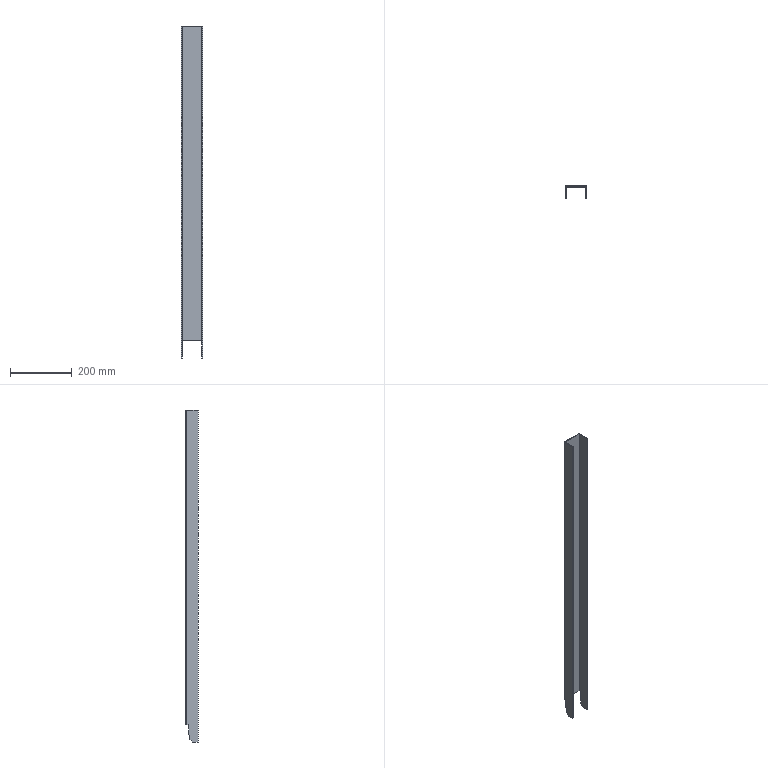Part | SolidWorks | 1 solid | 30 faces | box 70 x 40 x 1074 mm | volume 445087 mm3 | plane 26 | cylinder 4 | commonest cylinder face diameters 0.2 x2 6.2 x2
STEP:
#1=CARTESIAN_POINT('',(-31.9,-3.,-480.25));
#2=VERTEX_POINT('',#1);
#3=CARTESIAN_POINT('',(31.9,-3.,-480.25));
#4=VERTEX_POINT('',#3);
#5=CARTESIAN_POINT('',(0.,-3.,-480.25));
#6=DIRECTION('',(1.,0.,0.));
#7=VECTOR('',#6,1000.);
#8=LINE('',#5,#7);
#9=EDGE_CURVE('',#2,#4,#8,.T.);
#10=ORIENTED_EDGE('',*,*,#9,.T.);
#11=CARTESIAN_POINT('',(31.9,-3.,536.75));
#12=VERTEX_POINT('',#11);
#13=CARTESIAN_POINT('',(31.9,-3.,536.75));
#14=DIRECTION('',(0.,0.,-1.));
#15=VECTOR('',#14,1000.);
#16=LINE('',#13,#15);
#17=EDGE_CURVE('',#12,#4,#16,.T.);
#18=ORIENTED_EDGE('',*,*,#17,.F.);
#19=CARTESIAN_POINT('',(-31.9,-3.,536.75));
#20=VERTEX_POINT('',#19);
#21=CARTESIAN_POINT('',(35.,-3.,536.75));
#22=DIRECTION('',(1.,0.,0.));
#23=VECTOR('',#22,1000.);
#24=LINE('',#21,#23);
#25=EDGE_CURVE('',#20,#12,#24,.T.);
#26=ORIENTED_EDGE('',*,*,#25,.F.);
#27=CARTESIAN_POINT('',(-31.9,-3.,-536.75));
#28=DIRECTION('',(0.,0.,1.));
#29=VECTOR('',#28,1000.);
#30=LINE('',#27,#29);
#31=EDGE_CURVE('',#2,#20,#30,.T.);
#32=ORIENTED_EDGE('',*,*,#31,.F.);
#33=EDGE_LOOP('',(#10,#18,#26,#32));
#34=FACE_OUTER_BOUND('',#33,.T.);
#35=CARTESIAN_POINT('',(0.,-3.,0.));
#36=DIRECTION('',(0.,1.,0.));
#37=DIRECTION('',(0.,0.,1.));
#38=AXIS2_PLACEMENT_3D('',#35,#36,#37);
#39=PLANE('',#38);
#40=ADVANCED_FACE('',(#34),#39,.F.);
#41=CARTESIAN_POINT('',(31.9,0.,536.75));
#42=VERTEX_POINT('',#41);
#43=CARTESIAN_POINT('',(31.9,0.,-480.25));
#44=VERTEX_POINT('',#43);
#45=CARTESIAN_POINT('',(31.9,0.,536.75));
#46=DIRECTION('',(0.,0.,-1.));
#47=VECTOR('',#46,1000.);
#48=LINE('',#45,#47);
#49=EDGE_CURVE('',#42,#44,#48,.T.);
#50=ORIENTED_EDGE('',*,*,#49,.T.);
#51=CARTESIAN_POINT('',(-31.9,0.,-480.25));
#52=VERTEX_POINT('',#51);
#53=CARTESIAN_POINT('',(0.,0.,-480.25));
#54=DIRECTION('',(1.,0.,0.));
#55=VECTOR('',#54,1000.);
#56=LINE('',#53,#55);
#57=EDGE_CURVE('',#52,#44,#56,.T.);
#58=ORIENTED_EDGE('',*,*,#57,.F.);
#59=CARTESIAN_POINT('',(-31.9,0.,536.75));
#60=VERTEX_POINT('',#59);
#61=CARTESIAN_POINT('',(-31.9,0.,-536.75));
#62=DIRECTION('',(0.,0.,1.));
#63=VECTOR('',#62,1000.);
#64=LINE('',#61,#63);
#65=EDGE_CURVE('',#52,#60,#64,.T.);
#66=ORIENTED_EDGE('',*,*,#65,.T.);
#67=CARTESIAN_POINT('',(35.,0.,536.75));
#68=DIRECTION('',(1.,0.,0.));
#69=VECTOR('',#68,1000.);
#70=LINE('',#67,#69);
#71=EDGE_CURVE('',#60,#42,#70,.T.);
#72=ORIENTED_EDGE('',*,*,#71,.T.);
#73=EDGE_LOOP('',(#50,#58,#66,#72));
#74=FACE_OUTER_BOUND('',#73,.T.);
#75=CARTESIAN_POINT('',(0.,0.,0.));
#76=DIRECTION('',(0.,1.,0.));
#77=DIRECTION('',(0.,0.,1.));
#78=AXIS2_PLACEMENT_3D('',#75,#76,#77);
#79=PLANE('',#78);
#80=ADVANCED_FACE('',(#74),#79,.T.);
#81=ORIENTED_EDGE('',*,*,#65,.F.);
#82=CARTESIAN_POINT('',(-35.,-3.1,-480.25));
#83=VERTEX_POINT('',#82);
#84=CARTESIAN_POINT('',(-31.9,-3.1,-480.25));
#85=DIRECTION('',(0.,0.,-1.));
#86=DIRECTION('',(0.,-1.,0.));
#87=AXIS2_PLACEMENT_3D('',#84,#85,#86);
#88=CIRCLE('',#87,3.1);
#89=EDGE_CURVE('',#83,#52,#88,.T.);
#90=ORIENTED_EDGE('',*,*,#89,.F.);
#91=CARTESIAN_POINT('',(-35.,-3.1,536.75));
#92=VERTEX_POINT('',#91);
#93=CARTESIAN_POINT('',(-35.,-3.1,536.75));
#94=DIRECTION('',(0.,0.,1.));
#95=VECTOR('',#94,1000.);
#96=LINE('',#93,#95);
#97=EDGE_CURVE('',#83,#92,#96,.T.);
#98=ORIENTED_EDGE('',*,*,#97,.T.);
#99=CARTESIAN_POINT('',(-31.9,-3.1,536.75));
#100=DIRECTION('',(0.,0.,1.));
#101=DIRECTION('',(-1.,0.,0.));
#102=AXIS2_PLACEMENT_3D('',#99,#100,#101);
#103=CIRCLE('',#102,3.1);
#104=EDGE_CURVE('',#60,#92,#103,.T.);
#105=ORIENTED_EDGE('',*,*,#104,.F.);
#106=EDGE_LOOP('',(#81,#90,#98,#105));
#107=FACE_OUTER_BOUND('',#106,.T.);
#108=CARTESIAN_POINT('',(-31.9,-3.1,-536.75));
#109=DIRECTION('',(0.,0.,-1.));
#110=DIRECTION('',(-1.,0.,0.));
#111=AXIS2_PLACEMENT_3D('',#108,#109,#110);
#112=CYLINDRICAL_SURFACE('',#111,3.1);
#113=ADVANCED_FACE('',(#107),#112,.T.);
#114=CARTESIAN_POINT('',(-32.,-3.1,-480.25));
#115=VERTEX_POINT('',#114);
#116=CARTESIAN_POINT('',(-31.9,-3.1,-480.25));
#117=DIRECTION('',(0.,0.,-1.));
#118=DIRECTION('',(-1.,0.,0.));
#119=AXIS2_PLACEMENT_3D('',#116,#117,#118);
#120=CIRCLE('',#119,0.1);
#121=EDGE_CURVE('',#115,#2,#120,.T.);
#122=ORIENTED_EDGE('',*,*,#121,.T.);
#123=ORIENTED_EDGE('',*,*,#31,.T.);
#124=CARTESIAN_POINT('',(-32.,-3.1,536.75));
#125=VERTEX_POINT('',#124);
#126=CARTESIAN_POINT('',(-31.9,-3.1,536.75));
#127=DIRECTION('',(0.,0.,1.));
#128=DIRECTION('',(-1.,0.,0.));
#129=AXIS2_PLACEMENT_3D('',#126,#127,#128);
#130=CIRCLE('',#129,0.1);
#131=EDGE_CURVE('',#20,#125,#130,.T.);
#132=ORIENTED_EDGE('',*,*,#131,.T.);
#133=CARTESIAN_POINT('',(-32.,-3.1,536.75));
#134=DIRECTION('',(0.,0.,-1.));
#135=VECTOR('',#134,1000.);
#136=LINE('',#133,#135);
#137=EDGE_CURVE('',#125,#115,#136,.T.);
#138=ORIENTED_EDGE('',*,*,#137,.T.);
#139=EDGE_LOOP('',(#122,#123,#132,#138));
#140=FACE_OUTER_BOUND('',#139,.T.);
#141=CARTESIAN_POINT('',(-31.9,-3.1,-536.75));
#142=DIRECTION('',(0.,0.,-1.));
#143=DIRECTION('',(-1.,0.,0.));
#144=AXIS2_PLACEMENT_3D('',#141,#142,#143);
#145=CYLINDRICAL_SURFACE('',#144,0.1);
#146=ADVANCED_FACE('',(#140),#145,.F.);
#147=CARTESIAN_POINT('',(-32.,-21.55,-536.75));
#148=VERTEX_POINT('',#147);
#149=CARTESIAN_POINT('',(-35.,-21.55,-536.75));
#150=VERTEX_POINT('',#149);
#151=CARTESIAN_POINT('',(-32.,-21.55,-536.75));
#152=DIRECTION('',(-1.,0.,0.));
#153=VECTOR('',#152,1000.);
#154=LINE('',#151,#153);
#155=EDGE_CURVE('',#148,#150,#154,.T.);
#156=ORIENTED_EDGE('',*,*,#155,.F.);
#157=CARTESIAN_POINT('',(-32.,-40.,-536.75));
#158=VERTEX_POINT('',#157);
#159=CARTESIAN_POINT('',(-32.,-40.,-536.75));
#160=DIRECTION('',(0.,-1.,0.));
#161=VECTOR('',#160,1000.);
#162=LINE('',#159,#161);
#163=EDGE_CURVE('',#148,#158,#162,.T.);
#164=ORIENTED_EDGE('',*,*,#163,.T.);
#165=CARTESIAN_POINT('',(-35.,-40.,-536.75));
#166=VERTEX_POINT('',#165);
#167=CARTESIAN_POINT('',(-35.,-40.,-536.75));
#168=DIRECTION('',(1.,0.,0.));
#169=VECTOR('',#168,1000.);
#170=LINE('',#167,#169);
#171=EDGE_CURVE('',#166,#158,#170,.T.);
#172=ORIENTED_EDGE('',*,*,#171,.F.);
#173=CARTESIAN_POINT('',(-35.,0.,-536.75));
#174=DIRECTION('',(0.,-1.,0.));
#175=VECTOR('',#174,1000.);
#176=LINE('',#173,#175);
#177=EDGE_CURVE('',#150,#166,#176,.T.);
#178=ORIENTED_EDGE('',*,*,#177,.F.);
#179=EDGE_LOOP('',(#156,#164,#172,#178));
#180=FACE_OUTER_BOUND('',#179,.T.);
#181=CARTESIAN_POINT('',(-35.,-40.,-536.75));
#182=DIRECTION('',(0.,0.,1.));
#183=DIRECTION('',(1.,0.,0.));
#184=AXIS2_PLACEMENT_3D('',#181,#182,#183);
#185=PLANE('',#184);
#186=ADVANCED_FACE('',(#180),#185,.F.);
#187=CARTESIAN_POINT('',(-35.,-7.501,-480.25));
#188=VERTEX_POINT('',#187);
#189=CARTESIAN_POINT('',(-35.,0.,-480.25));
#190=DIRECTION('',(0.,-1.,0.));
#191=VECTOR('',#190,1000.);
#192=LINE('',#189,#191);
#193=EDGE_CURVE('',#83,#188,#192,.T.);
#194=ORIENTED_EDGE('',*,*,#193,.T.);
#195=CARTESIAN_POINT('',(-35.,-7.501,-484.727));
#196=VERTEX_POINT('',#195);
#197=CARTESIAN_POINT('',(-35.,-7.501,0.));
#198=DIRECTION('',(0.,0.,-1.));
#199=VECTOR('',#198,1000.);
#200=LINE('',#197,#199);
#201=EDGE_CURVE('',#188,#196,#200,.T.);
#202=ORIENTED_EDGE('',*,*,#201,.T.);
#203=CARTESIAN_POINT('',(-35.,-12.028,-527.795));
#204=VERTEX_POINT('',#203);
#205=CARTESIAN_POINT('',(-35.,42.971,-4.516));
#206=DIRECTION('',(0.,-0.1045,-0.9945));
#207=VECTOR('',#206,1000.);
#208=LINE('',#205,#207);
#209=EDGE_CURVE('',#196,#204,#208,.T.);
#210=ORIENTED_EDGE('',*,*,#209,.T.);
#211=CARTESIAN_POINT('',(-35.,257.756,-274.084));
#212=DIRECTION('',(0.,-0.7285,-0.6851));
#213=VECTOR('',#212,1000.);
#214=LINE('',#211,#213);
#215=EDGE_CURVE('',#204,#150,#214,.T.);
#216=ORIENTED_EDGE('',*,*,#215,.T.);
#217=ORIENTED_EDGE('',*,*,#177,.T.);
#218=CARTESIAN_POINT('',(-35.,-40.,536.75));
#219=VERTEX_POINT('',#218);
#220=CARTESIAN_POINT('',(-35.,-40.,0.));
#221=DIRECTION('',(0.,0.,1.));
#222=VECTOR('',#221,1000.);
#223=LINE('',#220,#222);
#224=EDGE_CURVE('',#166,#219,#223,.T.);
#225=ORIENTED_EDGE('',*,*,#224,.T.);
#226=CARTESIAN_POINT('',(-35.,0.,536.75));
#227=DIRECTION('',(0.,1.,0.));
#228=VECTOR('',#227,1000.);
#229=LINE('',#226,#228);
#230=EDGE_CURVE('',#219,#92,#229,.T.);
#231=ORIENTED_EDGE('',*,*,#230,.T.);
#232=ORIENTED_EDGE('',*,*,#97,.F.);
#233=EDGE_LOOP('',(#194,#202,#210,#216,#217,#225,#231,#232));
#234=FACE_OUTER_BOUND('',#233,.T.);
#235=CARTESIAN_POINT('',(-35.,0.,0.));
#236=DIRECTION('',(1.,0.,0.));
#237=DIRECTION('',(0.,1.,0.));
#238=AXIS2_PLACEMENT_3D('',#235,#236,#237);
#239=PLANE('',#238);
#240=ADVANCED_FACE('',(#234),#239,.F.);
#241=CARTESIAN_POINT('',(-32.,-7.501,-480.25));
#242=VERTEX_POINT('',#241);
#243=CARTESIAN_POINT('',(-32.,-7.501,-484.727));
#244=VERTEX_POINT('',#243);
#245=CARTESIAN_POINT('',(-32.,-7.501,0.));
#246=DIRECTION('',(0.,0.,-1.));
#247=VECTOR('',#246,1000.);
#248=LINE('',#245,#247);
#249=EDGE_CURVE('',#242,#244,#248,.T.);
#250=ORIENTED_EDGE('',*,*,#249,.F.);
#251=CARTESIAN_POINT('',(-32.,0.,-480.25));
#252=DIRECTION('',(0.,-1.,0.));
#253=VECTOR('',#252,1000.);
#254=LINE('',#251,#253);
#255=EDGE_CURVE('',#115,#242,#254,.T.);
#256=ORIENTED_EDGE('',*,*,#255,.F.);
#257=ORIENTED_EDGE('',*,*,#137,.F.);
#258=CARTESIAN_POINT('',(-32.,-40.,536.75));
#259=VERTEX_POINT('',#258);
#260=CARTESIAN_POINT('',(-32.,-3.,536.75));
#261=DIRECTION('',(0.,1.,0.));
#262=VECTOR('',#261,1000.);
#263=LINE('',#260,#262);
#264=EDGE_CURVE('',#259,#125,#263,.T.);
#265=ORIENTED_EDGE('',*,*,#264,.F.);
#266=CARTESIAN_POINT('',(-32.,-40.,536.75));
#267=DIRECTION('',(0.,0.,1.));
#268=VECTOR('',#267,1000.);
#269=LINE('',#266,#268);
#270=EDGE_CURVE('',#158,#259,#269,.T.);
#271=ORIENTED_EDGE('',*,*,#270,.F.);
#272=ORIENTED_EDGE('',*,*,#163,.F.);
#273=CARTESIAN_POINT('',(-32.,-12.028,-527.795));
#274=VERTEX_POINT('',#273);
#275=CARTESIAN_POINT('',(-32.,257.756,-274.084));
#276=DIRECTION('',(0.,-0.7285,-0.6851));
#277=VECTOR('',#276,1000.);
#278=LINE('',#275,#277);
#279=EDGE_CURVE('',#274,#148,#278,.T.);
#280=ORIENTED_EDGE('',*,*,#279,.F.);
#281=CARTESIAN_POINT('',(-32.,42.971,-4.516));
#282=DIRECTION('',(0.,-0.1045,-0.9945));
#283=VECTOR('',#282,1000.);
#284=LINE('',#281,#283);
#285=EDGE_CURVE('',#244,#274,#284,.T.);
#286=ORIENTED_EDGE('',*,*,#285,.F.);
#287=EDGE_LOOP('',(#250,#256,#257,#265,#271,#272,#280,#286));
#288=FACE_OUTER_BOUND('',#287,.T.);
#289=CARTESIAN_POINT('',(-32.,0.,0.));
#290=DIRECTION('',(1.,0.,0.));
#291=DIRECTION('',(0.,1.,0.));
#292=AXIS2_PLACEMENT_3D('',#289,#290,#291);
#293=PLANE('',#292);
#294=ADVANCED_FACE('',(#288),#293,.T.);
#295=CARTESIAN_POINT('',(35.,-3.1,536.75));
#296=VERTEX_POINT('',#295);
#297=CARTESIAN_POINT('',(35.,-3.1,-480.25));
#298=VERTEX_POINT('',#297);
#299=CARTESIAN_POINT('',(35.,-3.1,-536.75));
#300=DIRECTION('',(0.,0.,-1.));
#301=VECTOR('',#300,1000.);
#302=LINE('',#299,#301);
#303=EDGE_CURVE('',#296,#298,#302,.T.);
#304=ORIENTED_EDGE('',*,*,#303,.T.);
#305=CARTESIAN_POINT('',(31.9,-3.1,-480.25));
#306=DIRECTION('',(0.,0.,-1.));
#307=DIRECTION('',(1.,0.,0.));
#308=AXIS2_PLACEMENT_3D('',#305,#306,#307);
#309=CIRCLE('',#308,3.1);
#310=EDGE_CURVE('',#44,#298,#309,.T.);
#311=ORIENTED_EDGE('',*,*,#310,.F.);
#312=ORIENTED_EDGE('',*,*,#49,.F.);
#313=CARTESIAN_POINT('',(31.9,-3.1,536.75));
#314=DIRECTION('',(0.,0.,1.));
#315=DIRECTION('',(1.,0.,0.));
#316=AXIS2_PLACEMENT_3D('',#313,#314,#315);
#317=CIRCLE('',#316,3.1);
#318=EDGE_CURVE('',#296,#42,#317,.T.);
#319=ORIENTED_EDGE('',*,*,#318,.F.);
#320=EDGE_LOOP('',(#304,#311,#312,#319));
#321=FACE_OUTER_BOUND('',#320,.T.);
#322=CARTESIAN_POINT('',(31.9,-3.1,536.75));
#323=DIRECTION('',(0.,0.,1.));
#324=DIRECTION('',(1.,0.,0.));
#325=AXIS2_PLACEMENT_3D('',#322,#323,#324);
#326=CYLINDRICAL_SURFACE('',#325,3.1);
#327=ADVANCED_FACE('',(#321),#326,.T.);
#328=CARTESIAN_POINT('',(32.,-3.1,-480.25));
#329=VERTEX_POINT('',#328);
#330=CARTESIAN_POINT('',(31.9,-3.1,-480.25));
#331=DIRECTION('',(0.,0.,-1.));
#332=DIRECTION('',(0.,-1.,0.));
#333=AXIS2_PLACEMENT_3D('',#330,#331,#332);
#334=CIRCLE('',#333,0.1);
#335=EDGE_CURVE('',#4,#329,#334,.T.);
#336=ORIENTED_EDGE('',*,*,#335,.T.);
#337=CARTESIAN_POINT('',(32.,-3.1,536.75));
#338=VERTEX_POINT('',#337);
#339=CARTESIAN_POINT('',(32.,-3.1,-536.75));
#340=DIRECTION('',(0.,0.,1.));
#341=VECTOR('',#340,1000.);
#342=LINE('',#339,#341);
#343=EDGE_CURVE('',#329,#338,#342,.T.);
#344=ORIENTED_EDGE('',*,*,#343,.T.);
#345=CARTESIAN_POINT('',(31.9,-3.1,536.75));
#346=DIRECTION('',(0.,0.,1.));
#347=DIRECTION('',(1.,0.,0.));
#348=AXIS2_PLACEMENT_3D('',#345,#346,#347);
#349=CIRCLE('',#348,0.1);
#350=EDGE_CURVE('',#338,#12,#349,.T.);
#351=ORIENTED_EDGE('',*,*,#350,.T.);
#352=ORIENTED_EDGE('',*,*,#17,.T.);
#353=EDGE_LOOP('',(#336,#344,#351,#352));
#354=FACE_OUTER_BOUND('',#353,.T.);
#355=CARTESIAN_POINT('',(31.9,-3.1,536.75));
#356=DIRECTION('',(0.,0.,1.));
#357=DIRECTION('',(1.,0.,0.));
#358=AXIS2_PLACEMENT_3D('',#355,#356,#357);
#359=CYLINDRICAL_SURFACE('',#358,0.1);
#360=ADVANCED_FACE('',(#354),#359,.F.);
#361=CARTESIAN_POINT('',(32.,-21.55,-536.75));
#362=VERTEX_POINT('',#361);
#363=CARTESIAN_POINT('',(35.,-21.55,-536.75));
#364=VERTEX_POINT('',#363);
#365=CARTESIAN_POINT('',(32.,-21.55,-536.75));
#366=DIRECTION('',(1.,0.,0.));
#367=VECTOR('',#366,1000.);
#368=LINE('',#365,#367);
#369=EDGE_CURVE('',#362,#364,#368,.T.);
#370=ORIENTED_EDGE('',*,*,#369,.T.);
#371=CARTESIAN_POINT('',(35.,-40.,-536.75));
#372=VERTEX_POINT('',#371);
#373=CARTESIAN_POINT('',(35.,0.,-536.75));
#374=DIRECTION('',(0.,1.,0.));
#375=VECTOR('',#374,1000.);
#376=LINE('',#373,#375);
#377=EDGE_CURVE('',#372,#364,#376,.T.);
#378=ORIENTED_EDGE('',*,*,#377,.F.);
#379=CARTESIAN_POINT('',(32.,-40.,-536.75));
#380=VERTEX_POINT('',#379);
#381=CARTESIAN_POINT('',(35.,-40.,-536.75));
#382=DIRECTION('',(-1.,0.,0.));
#383=VECTOR('',#382,1000.);
#384=LINE('',#381,#383);
#385=EDGE_CURVE('',#372,#380,#384,.T.);
#386=ORIENTED_EDGE('',*,*,#385,.T.);
#387=CARTESIAN_POINT('',(32.,-3.,-536.75));
#388=DIRECTION('',(0.,1.,0.));
#389=VECTOR('',#388,1000.);
#390=LINE('',#387,#389);
#391=EDGE_CURVE('',#380,#362,#390,.T.);
#392=ORIENTED_EDGE('',*,*,#391,.T.);
#393=EDGE_LOOP('',(#370,#378,#386,#392));
#394=FACE_OUTER_BOUND('',#393,.T.);
#395=CARTESIAN_POINT('',(35.,-3.,-536.75));
#396=DIRECTION('',(0.,0.,1.));
#397=DIRECTION('',(1.,0.,0.));
#398=AXIS2_PLACEMENT_3D('',#395,#396,#397);
#399=PLANE('',#398);
#400=ADVANCED_FACE('',(#394),#399,.F.);
#401=CARTESIAN_POINT('',(35.,-12.028,-527.795));
#402=VERTEX_POINT('',#401);
#403=CARTESIAN_POINT('',(35.,257.756,-274.084));
#404=DIRECTION('',(0.,0.7285,0.6851));
#405=VECTOR('',#404,1000.);
#406=LINE('',#403,#405);
#407=EDGE_CURVE('',#364,#402,#406,.T.);
#408=ORIENTED_EDGE('',*,*,#407,.T.);
#409=CARTESIAN_POINT('',(35.,-7.501,-484.727));
#410=VERTEX_POINT('',#409);
#411=CARTESIAN_POINT('',(35.,42.971,-4.516));
#412=DIRECTION('',(0.,0.1045,0.9945));
#413=VECTOR('',#412,1000.);
#414=LINE('',#411,#413);
#415=EDGE_CURVE('',#402,#410,#414,.T.);
#416=ORIENTED_EDGE('',*,*,#415,.T.);
#417=CARTESIAN_POINT('',(35.,-7.501,-480.25));
#418=VERTEX_POINT('',#417);
#419=CARTESIAN_POINT('',(35.,-7.501,0.));
#420=DIRECTION('',(0.,0.,1.));
#421=VECTOR('',#420,1000.);
#422=LINE('',#419,#421);
#423=EDGE_CURVE('',#410,#418,#422,.T.);
#424=ORIENTED_EDGE('',*,*,#423,.T.);
#425=CARTESIAN_POINT('',(35.,0.,-480.25));
#426=DIRECTION('',(0.,1.,0.));
#427=VECTOR('',#426,1000.);
#428=LINE('',#425,#427);
#429=EDGE_CURVE('',#418,#298,#428,.T.);
#430=ORIENTED_EDGE('',*,*,#429,.T.);
#431=ORIENTED_EDGE('',*,*,#303,.F.);
#432=CARTESIAN_POINT('',(35.,-40.,536.75));
#433=VERTEX_POINT('',#432);
#434=CARTESIAN_POINT('',(35.,0.,536.75));
#435=DIRECTION('',(0.,-1.,0.));
#436=VECTOR('',#435,1000.);
#437=LINE('',#434,#436);
#438=EDGE_CURVE('',#296,#433,#437,.T.);
#439=ORIENTED_EDGE('',*,*,#438,.T.);
#440=CARTESIAN_POINT('',(35.,-40.,0.));
#441=DIRECTION('',(0.,0.,-1.));
#442=VECTOR('',#441,1000.);
#443=LINE('',#440,#442);
#444=EDGE_CURVE('',#433,#372,#443,.T.);
#445=ORIENTED_EDGE('',*,*,#444,.T.);
#446=ORIENTED_EDGE('',*,*,#377,.T.);
#447=EDGE_LOOP('',(#408,#416,#424,#430,#431,#439,#445,#446));
#448=FACE_OUTER_BOUND('',#447,.T.);
#449=CARTESIAN_POINT('',(35.,0.,0.));
#450=DIRECTION('',(-1.,0.,0.));
#451=DIRECTION('',(0.,-1.,0.));
#452=AXIS2_PLACEMENT_3D('',#449,#450,#451);
#453=PLANE('',#452);
#454=ADVANCED_FACE('',(#448),#453,.F.);
#455=CARTESIAN_POINT('',(32.,-12.028,-527.795));
#456=VERTEX_POINT('',#455);
#457=CARTESIAN_POINT('',(32.,-7.501,-484.727));
#458=VERTEX_POINT('',#457);
#459=CARTESIAN_POINT('',(32.,42.971,-4.516));
#460=DIRECTION('',(0.,0.1045,0.9945));
#461=VECTOR('',#460,1000.);
#462=LINE('',#459,#461);
#463=EDGE_CURVE('',#456,#458,#462,.T.);
#464=ORIENTED_EDGE('',*,*,#463,.F.);
#465=CARTESIAN_POINT('',(32.,257.756,-274.084));
#466=DIRECTION('',(0.,0.7285,0.6851));
#467=VECTOR('',#466,1000.);
#468=LINE('',#465,#467);
#469=EDGE_CURVE('',#362,#456,#468,.T.);
#470=ORIENTED_EDGE('',*,*,#469,.F.);
#471=ORIENTED_EDGE('',*,*,#391,.F.);
#472=CARTESIAN_POINT('',(32.,-40.,536.75));
#473=VERTEX_POINT('',#472);
#474=CARTESIAN_POINT('',(32.,-40.,-536.75));
#475=DIRECTION('',(0.,0.,-1.));
#476=VECTOR('',#475,1000.);
#477=LINE('',#474,#476);
#478=EDGE_CURVE('',#473,#380,#477,.T.);
#479=ORIENTED_EDGE('',*,*,#478,.F.);
#480=CARTESIAN_POINT('',(32.,-40.,536.75));
#481=DIRECTION('',(0.,-1.,0.));
#482=VECTOR('',#481,1000.);
#483=LINE('',#480,#482);
#484=EDGE_CURVE('',#338,#473,#483,.T.);
#485=ORIENTED_EDGE('',*,*,#484,.F.);
#486=ORIENTED_EDGE('',*,*,#343,.F.);
#487=CARTESIAN_POINT('',(32.,-7.501,-480.25));
#488=VERTEX_POINT('',#487);
#489=CARTESIAN_POINT('',(32.,0.,-480.25));
#490=DIRECTION('',(0.,1.,0.));
#491=VECTOR('',#490,1000.);
#492=LINE('',#489,#491);
#493=EDGE_CURVE('',#488,#329,#492,.T.);
#494=ORIENTED_EDGE('',*,*,#493,.F.);
#495=CARTESIAN_POINT('',(32.,-7.501,0.));
#496=DIRECTION('',(0.,0.,1.));
#497=VECTOR('',#496,1000.);
#498=LINE('',#495,#497);
#499=EDGE_CURVE('',#458,#488,#498,.T.);
#500=ORIENTED_EDGE('',*,*,#499,.F.);
#501=EDGE_LOOP('',(#464,#470,#471,#479,#485,#486,#494,#500));
#502=FACE_OUTER_BOUND('',#501,.T.);
#503=CARTESIAN_POINT('',(32.,0.,0.));
#504=DIRECTION('',(-1.,0.,0.));
#505=DIRECTION('',(0.,-1.,0.));
#506=AXIS2_PLACEMENT_3D('',#503,#504,#505);
#507=PLANE('',#506);
#508=ADVANCED_FACE('',(#502),#507,.T.);
#509=ORIENTED_EDGE('',*,*,#25,.T.);
#510=CARTESIAN_POINT('',(31.9,-3.,536.75));
#511=DIRECTION('',(0.,1.,0.));
#512=VECTOR('',#511,1000.);
#513=LINE('',#510,#512);
#514=EDGE_CURVE('',#12,#42,#513,.T.);
#515=ORIENTED_EDGE('',*,*,#514,.T.);
#516=ORIENTED_EDGE('',*,*,#71,.F.);
#517=CARTESIAN_POINT('',(-31.9,-3.,536.75));
#518=DIRECTION('',(0.,1.,0.));
#519=VECTOR('',#518,1000.);
#520=LINE('',#517,#519);
#521=EDGE_CURVE('',#20,#60,#520,.T.);
#522=ORIENTED_EDGE('',*,*,#521,.F.);
#523=EDGE_LOOP('',(#509,#515,#516,#522));
#524=FACE_OUTER_BOUND('',#523,.T.);
#525=CARTESIAN_POINT('',(35.,-3.,536.75));
#526=DIRECTION('',(0.,0.,1.));
#527=DIRECTION('',(1.,0.,0.));
#528=AXIS2_PLACEMENT_3D('',#525,#526,#527);
#529=PLANE('',#528);
#530=ADVANCED_FACE('',(#524),#529,.T.);
#531=CARTESIAN_POINT('',(-35.,-3.1,536.75));
#532=DIRECTION('',(-1.,0.,0.));
#533=VECTOR('',#532,1000.);
#534=LINE('',#531,#533);
#535=EDGE_CURVE('',#125,#92,#534,.T.);
#536=ORIENTED_EDGE('',*,*,#535,.F.);
#537=ORIENTED_EDGE('',*,*,#131,.F.);
#538=ORIENTED_EDGE('',*,*,#521,.T.);
#539=ORIENTED_EDGE('',*,*,#104,.T.);
#540=EDGE_LOOP('',(#536,#537,#538,#539));
#541=FACE_OUTER_BOUND('',#540,.T.);
#542=CARTESIAN_POINT('',(-31.9,-3.1,536.75));
#543=DIRECTION('',(0.,0.,1.));
#544=DIRECTION('',(1.,0.,0.));
#545=AXIS2_PLACEMENT_3D('',#542,#543,#544);
#546=PLANE('',#545);
#547=ADVANCED_FACE('',(#541),#546,.T.);
#548=ORIENTED_EDGE('',*,*,#535,.T.);
#549=ORIENTED_EDGE('',*,*,#230,.F.);
#550=CARTESIAN_POINT('',(-35.,-40.,536.75));
#551=DIRECTION('',(1.,0.,0.));
#552=VECTOR('',#551,1000.);
#553=LINE('',#550,#552);
#554=EDGE_CURVE('',#219,#259,#553,.T.);
#555=ORIENTED_EDGE('',*,*,#554,.T.);
#556=ORIENTED_EDGE('',*,*,#264,.T.);
#557=EDGE_LOOP('',(#548,#549,#555,#556));
#558=FACE_OUTER_BOUND('',#557,.T.);
#559=CARTESIAN_POINT('',(-35.,-3.,536.75));
#560=DIRECTION('',(0.,0.,-1.));
#561=DIRECTION('',(-1.,0.,0.));
#562=AXIS2_PLACEMENT_3D('',#559,#560,#561);
#563=PLANE('',#562);
#564=ADVANCED_FACE('',(#558),#563,.F.);
#565=ORIENTED_EDGE('',*,*,#270,.T.);
#566=ORIENTED_EDGE('',*,*,#554,.F.);
#567=ORIENTED_EDGE('',*,*,#224,.F.);
#568=ORIENTED_EDGE('',*,*,#171,.T.);
#569=EDGE_LOOP('',(#565,#566,#567,#568));
#570=FACE_OUTER_BOUND('',#569,.T.);
#571=CARTESIAN_POINT('',(-35.,-40.,536.75));
#572=DIRECTION('',(0.,1.,0.));
#573=DIRECTION('',(-1.,0.,0.));
#574=AXIS2_PLACEMENT_3D('',#571,#572,#573);
#575=PLANE('',#574);
#576=ADVANCED_FACE('',(#570),#575,.F.);
#577=ORIENTED_EDGE('',*,*,#350,.F.);
#578=CARTESIAN_POINT('',(32.,-3.1,536.75));
#579=DIRECTION('',(1.,0.,0.));
#580=VECTOR('',#579,1000.);
#581=LINE('',#578,#580);
#582=EDGE_CURVE('',#338,#296,#581,.T.);
#583=ORIENTED_EDGE('',*,*,#582,.T.);
#584=ORIENTED_EDGE('',*,*,#318,.T.);
#585=ORIENTED_EDGE('',*,*,#514,.F.);
#586=EDGE_LOOP('',(#577,#583,#584,#585));
#587=FACE_OUTER_BOUND('',#586,.T.);
#588=CARTESIAN_POINT('',(31.9,-3.1,536.75));
#589=DIRECTION('',(0.,0.,-1.));
#590=DIRECTION('',(-1.,0.,0.));
#591=AXIS2_PLACEMENT_3D('',#588,#589,#590);
#592=PLANE('',#591);
#593=ADVANCED_FACE('',(#587),#592,.F.);
#594=ORIENTED_EDGE('',*,*,#582,.F.);
#595=ORIENTED_EDGE('',*,*,#484,.T.);
#596=CARTESIAN_POINT('',(35.,-40.,536.75));
#597=DIRECTION('',(-1.,0.,0.));
#598=VECTOR('',#597,1000.);
#599=LINE('',#596,#598);
#600=EDGE_CURVE('',#433,#473,#599,.T.);
#601=ORIENTED_EDGE('',*,*,#600,.F.);
#602=ORIENTED_EDGE('',*,*,#438,.F.);
#603=EDGE_LOOP('',(#594,#595,#601,#602));
#604=FACE_OUTER_BOUND('',#603,.T.);
#605=CARTESIAN_POINT('',(35.,-40.,536.75));
#606=DIRECTION('',(0.,0.,-1.));
#607=DIRECTION('',(-1.,0.,0.));
#608=AXIS2_PLACEMENT_3D('',#605,#606,#607);
#609=PLANE('',#608);
#610=ADVANCED_FACE('',(#604),#609,.F.);
#611=ORIENTED_EDGE('',*,*,#478,.T.);
#612=ORIENTED_EDGE('',*,*,#385,.F.);
#613=ORIENTED_EDGE('',*,*,#444,.F.);
#614=ORIENTED_EDGE('',*,*,#600,.T.);
#615=EDGE_LOOP('',(#611,#612,#613,#614));
#616=FACE_OUTER_BOUND('',#615,.T.);
#617=CARTESIAN_POINT('',(35.,-40.,-536.75));
#618=DIRECTION('',(0.,1.,0.));
#619=DIRECTION('',(-1.,0.,0.));
#620=AXIS2_PLACEMENT_3D('',#617,#618,#619);
#621=PLANE('',#620);
#622=ADVANCED_FACE('',(#616),#621,.F.);
#623=CARTESIAN_POINT('',(-32.,-3.1,-480.25));
#624=DIRECTION('',(-1.,0.,0.));
#625=VECTOR('',#624,1000.);
#626=LINE('',#623,#625);
#627=EDGE_CURVE('',#115,#83,#626,.T.);
#628=ORIENTED_EDGE('',*,*,#627,.F.);
#629=ORIENTED_EDGE('',*,*,#255,.T.);
#630=CARTESIAN_POINT('',(-32.,-7.501,-480.25));
#631=DIRECTION('',(-1.,0.,0.));
#632=VECTOR('',#631,1000.);
#633=LINE('',#630,#632);
#634=EDGE_CURVE('',#242,#188,#633,.T.);
#635=ORIENTED_EDGE('',*,*,#634,.T.);
#636=ORIENTED_EDGE('',*,*,#193,.F.);
#637=EDGE_LOOP('',(#628,#629,#635,#636));
#638=FACE_OUTER_BOUND('',#637,.T.);
#639=CARTESIAN_POINT('',(-32.,0.,-480.25));
#640=DIRECTION('',(0.,0.,1.));
#641=DIRECTION('',(0.,-1.,0.));
#642=AXIS2_PLACEMENT_3D('',#639,#640,#641);
#643=PLANE('',#642);
#644=ADVANCED_FACE('',(#638),#643,.F.);
#645=ORIENTED_EDGE('',*,*,#634,.F.);
#646=ORIENTED_EDGE('',*,*,#249,.T.);
#647=CARTESIAN_POINT('',(-32.,-7.501,-484.727));
#648=DIRECTION('',(-1.,0.,0.));
#649=VECTOR('',#648,1000.);
#650=LINE('',#647,#649);
#651=EDGE_CURVE('',#244,#196,#650,.T.);
#652=ORIENTED_EDGE('',*,*,#651,.T.);
#653=ORIENTED_EDGE('',*,*,#201,.F.);
#654=EDGE_LOOP('',(#645,#646,#652,#653));
#655=FACE_OUTER_BOUND('',#654,.T.);
#656=CARTESIAN_POINT('',(-32.,-7.501,0.));
#657=DIRECTION('',(0.,-1.,0.));
#658=DIRECTION('',(0.,0.,-1.));
#659=AXIS2_PLACEMENT_3D('',#656,#657,#658);
#660=PLANE('',#659);
#661=ADVANCED_FACE('',(#655),#660,.F.);
#662=ORIENTED_EDGE('',*,*,#651,.F.);
#663=ORIENTED_EDGE('',*,*,#285,.T.);
#664=CARTESIAN_POINT('',(-32.,-12.028,-527.795));
#665=DIRECTION('',(-1.,0.,0.));
#666=VECTOR('',#665,1000.);
#667=LINE('',#664,#666);
#668=EDGE_CURVE('',#274,#204,#667,.T.);
#669=ORIENTED_EDGE('',*,*,#668,.T.);
#670=ORIENTED_EDGE('',*,*,#209,.F.);
#671=EDGE_LOOP('',(#662,#663,#669,#670));
#672=FACE_OUTER_BOUND('',#671,.T.);
#673=CARTESIAN_POINT('',(-32.,42.971,-4.516));
#674=DIRECTION('',(0.,-0.9945,0.1045));
#675=DIRECTION('',(0.,-0.1045,-0.9945));
#676=AXIS2_PLACEMENT_3D('',#673,#674,#675);
#677=PLANE('',#676);
#678=ADVANCED_FACE('',(#672),#677,.F.);
#679=ORIENTED_EDGE('',*,*,#279,.T.);
#680=ORIENTED_EDGE('',*,*,#155,.T.);
#681=ORIENTED_EDGE('',*,*,#215,.F.);
#682=ORIENTED_EDGE('',*,*,#668,.F.);
#683=EDGE_LOOP('',(#679,#680,#681,#682));
#684=FACE_OUTER_BOUND('',#683,.T.);
#685=CARTESIAN_POINT('',(-32.,257.756,-274.084));
#686=DIRECTION('',(0.,-0.6851,0.7285));
#687=DIRECTION('',(0.,-0.7285,-0.6851));
#688=AXIS2_PLACEMENT_3D('',#685,#686,#687);
#689=PLANE('',#688);
#690=ADVANCED_FACE('',(#684),#689,.F.);
#691=ORIENTED_EDGE('',*,*,#369,.F.);
#692=ORIENTED_EDGE('',*,*,#469,.T.);
#693=CARTESIAN_POINT('',(32.,-12.028,-527.795));
#694=DIRECTION('',(1.,0.,0.));
#695=VECTOR('',#694,1000.);
#696=LINE('',#693,#695);
#697=EDGE_CURVE('',#456,#402,#696,.T.);
#698=ORIENTED_EDGE('',*,*,#697,.T.);
#699=ORIENTED_EDGE('',*,*,#407,.F.);
#700=EDGE_LOOP('',(#691,#692,#698,#699));
#701=FACE_OUTER_BOUND('',#700,.T.);
#702=CARTESIAN_POINT('',(32.,257.756,-274.084));
#703=DIRECTION('',(0.,-0.6851,0.7285));
#704=DIRECTION('',(0.,0.7285,0.6851));
#705=AXIS2_PLACEMENT_3D('',#702,#703,#704);
#706=PLANE('',#705);
#707=ADVANCED_FACE('',(#701),#706,.F.);
#708=ORIENTED_EDGE('',*,*,#697,.F.);
#709=ORIENTED_EDGE('',*,*,#463,.T.);
#710=CARTESIAN_POINT('',(32.,-7.501,-484.727));
#711=DIRECTION('',(1.,0.,0.));
#712=VECTOR('',#711,1000.);
#713=LINE('',#710,#712);
#714=EDGE_CURVE('',#458,#410,#713,.T.);
#715=ORIENTED_EDGE('',*,*,#714,.T.);
#716=ORIENTED_EDGE('',*,*,#415,.F.);
#717=EDGE_LOOP('',(#708,#709,#715,#716));
#718=FACE_OUTER_BOUND('',#717,.T.);
#719=CARTESIAN_POINT('',(32.,42.971,-4.516));
#720=DIRECTION('',(0.,-0.9945,0.1045));
#721=DIRECTION('',(0.,0.1045,0.9945));
#722=AXIS2_PLACEMENT_3D('',#719,#720,#721);
#723=PLANE('',#722);
#724=ADVANCED_FACE('',(#718),#723,.F.);
#725=ORIENTED_EDGE('',*,*,#714,.F.);
#726=ORIENTED_EDGE('',*,*,#499,.T.);
#727=CARTESIAN_POINT('',(32.,-7.501,-480.25));
#728=DIRECTION('',(1.,0.,0.));
#729=VECTOR('',#728,1000.);
#730=LINE('',#727,#729);
#731=EDGE_CURVE('',#488,#418,#730,.T.);
#732=ORIENTED_EDGE('',*,*,#731,.T.);
#733=ORIENTED_EDGE('',*,*,#423,.F.);
#734=EDGE_LOOP('',(#725,#726,#732,#733));
#735=FACE_OUTER_BOUND('',#734,.T.);
#736=CARTESIAN_POINT('',(32.,-7.501,0.));
#737=DIRECTION('',(0.,-1.,0.));
#738=DIRECTION('',(0.,0.,1.));
#739=AXIS2_PLACEMENT_3D('',#736,#737,#738);
#740=PLANE('',#739);
#741=ADVANCED_FACE('',(#735),#740,.F.);
#742=ORIENTED_EDGE('',*,*,#493,.T.);
#743=CARTESIAN_POINT('',(32.,-3.1,-480.25));
#744=DIRECTION('',(1.,0.,0.));
#745=VECTOR('',#744,1000.);
#746=LINE('',#743,#745);
#747=EDGE_CURVE('',#329,#298,#746,.T.);
#748=ORIENTED_EDGE('',*,*,#747,.T.);
#749=ORIENTED_EDGE('',*,*,#429,.F.);
#750=ORIENTED_EDGE('',*,*,#731,.F.);
#751=EDGE_LOOP('',(#742,#748,#749,#750));
#752=FACE_OUTER_BOUND('',#751,.T.);
#753=CARTESIAN_POINT('',(32.,0.,-480.25));
#754=DIRECTION('',(0.,0.,1.));
#755=DIRECTION('',(0.,1.,0.));
#756=AXIS2_PLACEMENT_3D('',#753,#754,#755);
#757=PLANE('',#756);
#758=ADVANCED_FACE('',(#752),#757,.F.);
#759=ORIENTED_EDGE('',*,*,#747,.F.);
#760=ORIENTED_EDGE('',*,*,#335,.F.);
#761=CARTESIAN_POINT('',(31.9,-3.,-480.25));
#762=DIRECTION('',(0.,1.,0.));
#763=VECTOR('',#762,1000.);
#764=LINE('',#761,#763);
#765=EDGE_CURVE('',#4,#44,#764,.T.);
#766=ORIENTED_EDGE('',*,*,#765,.T.);
#767=ORIENTED_EDGE('',*,*,#310,.T.);
#768=EDGE_LOOP('',(#759,#760,#766,#767));
#769=FACE_OUTER_BOUND('',#768,.T.);
#770=CARTESIAN_POINT('',(31.9,-3.1,-480.25));
#771=DIRECTION('',(0.,0.,-1.));
#772=DIRECTION('',(0.,1.,0.));
#773=AXIS2_PLACEMENT_3D('',#770,#771,#772);
#774=PLANE('',#773);
#775=ADVANCED_FACE('',(#769),#774,.T.);
#776=ORIENTED_EDGE('',*,*,#765,.F.);
#777=ORIENTED_EDGE('',*,*,#9,.F.);
#778=CARTESIAN_POINT('',(-31.9,-3.,-480.25));
#779=DIRECTION('',(0.,1.,0.));
#780=VECTOR('',#779,1000.);
#781=LINE('',#778,#780);
#782=EDGE_CURVE('',#2,#52,#781,.T.);
#783=ORIENTED_EDGE('',*,*,#782,.T.);
#784=ORIENTED_EDGE('',*,*,#57,.T.);
#785=EDGE_LOOP('',(#776,#777,#783,#784));
#786=FACE_OUTER_BOUND('',#785,.T.);
#787=CARTESIAN_POINT('',(0.,-3.,-480.25));
#788=DIRECTION('',(0.,0.,1.));
#789=DIRECTION('',(1.,0.,0.));
#790=AXIS2_PLACEMENT_3D('',#787,#788,#789);
#791=PLANE('',#790);
#792=ADVANCED_FACE('',(#786),#791,.F.);
#793=ORIENTED_EDGE('',*,*,#89,.T.);
#794=ORIENTED_EDGE('',*,*,#782,.F.);
#795=ORIENTED_EDGE('',*,*,#121,.F.);
#796=ORIENTED_EDGE('',*,*,#627,.T.);
#797=EDGE_LOOP('',(#793,#794,#795,#796));
#798=FACE_OUTER_BOUND('',#797,.T.);
#799=CARTESIAN_POINT('',(-31.9,-3.1,-480.25));
#800=DIRECTION('',(0.,0.,-1.));
#801=DIRECTION('',(0.,1.,0.));
#802=AXIS2_PLACEMENT_3D('',#799,#800,#801);
#803=PLANE('',#802);
#804=ADVANCED_FACE('',(#798),#803,.T.);
#805=CLOSED_SHELL('',(#40,#80,#113,#146,#186,#240,#294,#327,#360,#400,#454,#508,#530,#547,#564,#576,#593,#610,#622,#644,#661,#678,#690,#707,#724,#741,#758,#775,#792,#804));
#806=MANIFOLD_SOLID_BREP('',#805);
#807=CARTESIAN_POINT('',(0.,0.,0.));
#808=DIRECTION('',(0.,0.,1.));
#809=DIRECTION('',(1.,0.,0.));
#810=AXIS2_PLACEMENT_3D('',#807,#808,#809);
#811=(LENGTH_UNIT()NAMED_UNIT(*)SI_UNIT(.MILLI.,.METRE.));
#812=UNCERTAINTY_MEASURE_WITH_UNIT(LENGTH_MEASURE(0.00001),#811,'','');
#813=(NAMED_UNIT(*)PLANE_ANGLE_UNIT()SI_UNIT($,.RADIAN.));
#814=(NAMED_UNIT(*)SI_UNIT($,.STERADIAN.)SOLID_ANGLE_UNIT());
#815=(GEOMETRIC_REPRESENTATION_CONTEXT(3)GLOBAL_UNCERTAINTY_ASSIGNED_CONTEXT((#812))GLOBAL_UNIT_ASSIGNED_CONTEXT((#811,#813,#814))REPRESENTATION_CONTEXT('',''));
#816=ADVANCED_BREP_SHAPE_REPRESENTATION('',(#806,#810),#815);